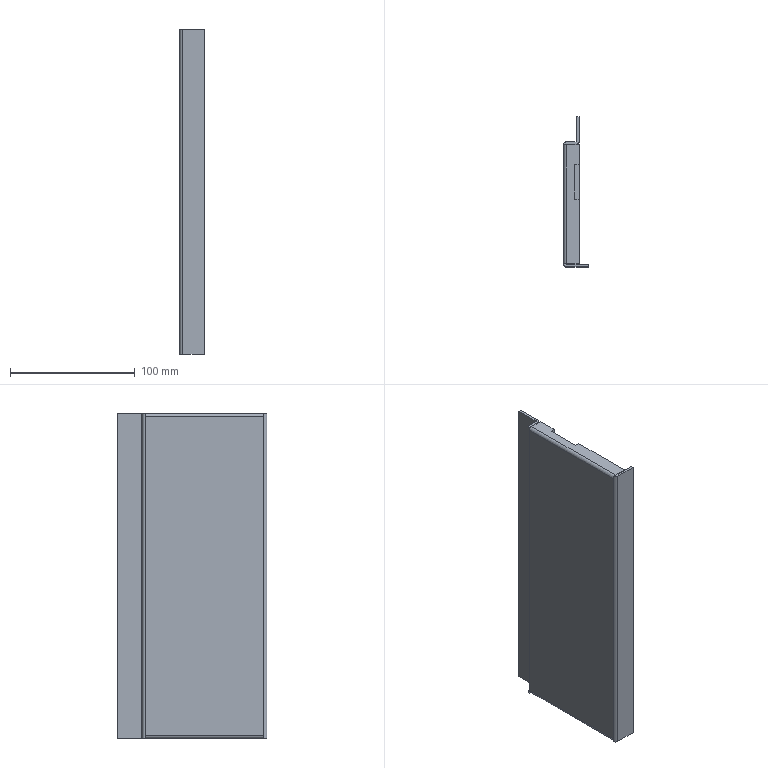Part | STEP file | Right Cover Plate | 1 solid | 42 faces | box 20 x 120 x 260 mm | volume 79765 mm3 | plane 32 | cylinder 10 | commonest cylinder face diameters 1 x5 5 x5
STEP:
#1=CARTESIAN_POINT('',(-10.5,-69.434,257.5));
#2=VERTEX_POINT('',#1);
#3=CARTESIAN_POINT('',(-10.5,-69.434,2.5));
#4=VERTEX_POINT('',#3);
#5=CARTESIAN_POINT('',(-10.5,-69.434,260.));
#6=DIRECTION('',(0.,0.,-1.));
#7=VECTOR('',#6,1000.);
#8=LINE('',#5,#7);
#9=EDGE_CURVE('',#2,#4,#8,.T.);
#10=ORIENTED_EDGE('',*,*,#9,.F.);
#11=CARTESIAN_POINT('',(-10.5,25.566,257.5));
#12=VERTEX_POINT('',#11);
#13=CARTESIAN_POINT('',(-10.5,28.066,257.5));
#14=DIRECTION('',(0.,-1.,0.));
#15=VECTOR('',#14,1000.);
#16=LINE('',#13,#15);
#17=EDGE_CURVE('',#12,#2,#16,.T.);
#18=ORIENTED_EDGE('',*,*,#17,.F.);
#19=CARTESIAN_POINT('',(-10.5,25.566,2.5));
#20=VERTEX_POINT('',#19);
#21=CARTESIAN_POINT('',(-10.5,25.566,260.));
#22=DIRECTION('',(0.,0.,1.));
#23=VECTOR('',#22,1000.);
#24=LINE('',#21,#23);
#25=EDGE_CURVE('',#20,#12,#24,.T.);
#26=ORIENTED_EDGE('',*,*,#25,.F.);
#27=CARTESIAN_POINT('',(-10.5,28.066,2.5));
#28=DIRECTION('',(0.,1.,0.));
#29=VECTOR('',#28,1000.);
#30=LINE('',#27,#29);
#31=EDGE_CURVE('',#4,#20,#30,.T.);
#32=ORIENTED_EDGE('',*,*,#31,.F.);
#33=EDGE_LOOP('',(#10,#18,#26,#32));
#34=FACE_OUTER_BOUND('',#33,.T.);
#35=CARTESIAN_POINT('',(-10.5,28.066,260.));
#36=DIRECTION('',(1.,0.,0.));
#37=DIRECTION('',(0.,1.,0.));
#38=AXIS2_PLACEMENT_3D('',#35,#36,#37);
#39=PLANE('',#38);
#40=ADVANCED_FACE('',(#34),#39,.F.);
#41=CARTESIAN_POINT('',(-8.5,-69.434,0.05051));
#42=VERTEX_POINT('',#41);
#43=CARTESIAN_POINT('',(-8.,-69.434,0.));
#44=VERTEX_POINT('',#43);
#45=CARTESIAN_POINT('',(-8.,-69.434,2.5));
#46=DIRECTION('',(0.,-1.,0.));
#47=DIRECTION('',(0.,0.,1.));
#48=AXIS2_PLACEMENT_3D('',#45,#46,#47);
#49=CIRCLE('',#48,2.5);
#50=EDGE_CURVE('',#42,#44,#49,.T.);
#51=ORIENTED_EDGE('',*,*,#50,.F.);
#52=CARTESIAN_POINT('',(-8.,-69.434,2.5));
#53=DIRECTION('',(0.,1.,0.));
#54=DIRECTION('',(0.,0.,1.));
#55=AXIS2_PLACEMENT_3D('',#52,#53,#54);
#56=CIRCLE('',#55,2.5);
#57=EDGE_CURVE('',#42,#4,#56,.T.);
#58=ORIENTED_EDGE('',*,*,#57,.T.);
#59=ORIENTED_EDGE('',*,*,#31,.T.);
#60=CARTESIAN_POINT('',(-8.5,25.566,0.05051));
#61=VERTEX_POINT('',#60);
#62=CARTESIAN_POINT('',(-8.,25.566,2.5));
#63=DIRECTION('',(0.,-1.,0.));
#64=DIRECTION('',(0.,0.,1.));
#65=AXIS2_PLACEMENT_3D('',#62,#63,#64);
#66=CIRCLE('',#65,2.5);
#67=EDGE_CURVE('',#20,#61,#66,.T.);
#68=ORIENTED_EDGE('',*,*,#67,.T.);
#69=CARTESIAN_POINT('',(-8.,25.566,0.));
#70=VERTEX_POINT('',#69);
#71=CARTESIAN_POINT('',(-8.,25.566,2.5));
#72=DIRECTION('',(0.,-1.,0.));
#73=DIRECTION('',(0.,0.,1.));
#74=AXIS2_PLACEMENT_3D('',#71,#72,#73);
#75=CIRCLE('',#74,2.5);
#76=EDGE_CURVE('',#61,#70,#75,.T.);
#77=ORIENTED_EDGE('',*,*,#76,.T.);
#78=CARTESIAN_POINT('',(-8.,25.566,0.));
#79=DIRECTION('',(0.,-1.,0.));
#80=VECTOR('',#79,1000.);
#81=LINE('',#78,#80);
#82=EDGE_CURVE('',#70,#44,#81,.T.);
#83=ORIENTED_EDGE('',*,*,#82,.T.);
#84=EDGE_LOOP('',(#51,#58,#59,#68,#77,#83));
#85=FACE_OUTER_BOUND('',#84,.T.);
#86=CARTESIAN_POINT('',(-8.,25.566,2.5));
#87=DIRECTION('',(0.,1.,0.));
#88=DIRECTION('',(0.,0.,1.));
#89=AXIS2_PLACEMENT_3D('',#86,#87,#88);
#90=CYLINDRICAL_SURFACE('',#89,2.5);
#91=ADVANCED_FACE('',(#85),#90,.T.);
#92=ORIENTED_EDGE('',*,*,#9,.T.);
#93=CARTESIAN_POINT('',(-10.5,-69.434,0.));
#94=VERTEX_POINT('',#93);
#95=CARTESIAN_POINT('',(-10.5,-69.434,260.));
#96=DIRECTION('',(0.,0.,-1.));
#97=VECTOR('',#96,1000.);
#98=LINE('',#95,#97);
#99=EDGE_CURVE('',#4,#94,#98,.T.);
#100=ORIENTED_EDGE('',*,*,#99,.T.);
#101=CARTESIAN_POINT('',(-8.,-71.934,0.));
#102=VERTEX_POINT('',#101);
#103=CARTESIAN_POINT('',(-8.,-69.434,0.));
#104=DIRECTION('',(0.,0.,1.));
#105=DIRECTION('',(-1.,0.,0.));
#106=AXIS2_PLACEMENT_3D('',#103,#104,#105);
#107=CIRCLE('',#106,2.5);
#108=EDGE_CURVE('',#94,#102,#107,.T.);
#109=ORIENTED_EDGE('',*,*,#108,.T.);
#110=CARTESIAN_POINT('',(-8.,-71.934,260.));
#111=VERTEX_POINT('',#110);
#112=CARTESIAN_POINT('',(-8.,-71.934,260.));
#113=DIRECTION('',(0.,0.,1.));
#114=VECTOR('',#113,1000.);
#115=LINE('',#112,#114);
#116=EDGE_CURVE('',#102,#111,#115,.T.);
#117=ORIENTED_EDGE('',*,*,#116,.T.);
#118=CARTESIAN_POINT('',(-10.5,-69.434,260.));
#119=VERTEX_POINT('',#118);
#120=CARTESIAN_POINT('',(-8.,-69.434,260.));
#121=DIRECTION('',(0.,0.,-1.));
#122=DIRECTION('',(-1.,0.,0.));
#123=AXIS2_PLACEMENT_3D('',#120,#121,#122);
#124=CIRCLE('',#123,2.5);
#125=EDGE_CURVE('',#111,#119,#124,.T.);
#126=ORIENTED_EDGE('',*,*,#125,.T.);
#127=CARTESIAN_POINT('',(-10.5,-69.434,260.));
#128=DIRECTION('',(0.,0.,-1.));
#129=VECTOR('',#128,1000.);
#130=LINE('',#127,#129);
#131=EDGE_CURVE('',#119,#2,#130,.T.);
#132=ORIENTED_EDGE('',*,*,#131,.T.);
#133=EDGE_LOOP('',(#92,#100,#109,#117,#126,#132));
#134=FACE_OUTER_BOUND('',#133,.T.);
#135=CARTESIAN_POINT('',(-8.,-69.434,260.));
#136=DIRECTION('',(0.,0.,-1.));
#137=DIRECTION('',(-1.,0.,0.));
#138=AXIS2_PLACEMENT_3D('',#135,#136,#137);
#139=CYLINDRICAL_SURFACE('',#138,2.5);
#140=ADVANCED_FACE('',(#134),#139,.T.);
#141=CARTESIAN_POINT('',(-8.5,25.566,259.949));
#142=VERTEX_POINT('',#141);
#143=CARTESIAN_POINT('',(-8.,25.566,260.));
#144=VERTEX_POINT('',#143);
#145=CARTESIAN_POINT('',(-8.,25.566,257.5));
#146=DIRECTION('',(0.,1.,0.));
#147=DIRECTION('',(0.,0.,-1.));
#148=AXIS2_PLACEMENT_3D('',#145,#146,#147);
#149=CIRCLE('',#148,2.5);
#150=EDGE_CURVE('',#142,#144,#149,.T.);
#151=ORIENTED_EDGE('',*,*,#150,.F.);
#152=CARTESIAN_POINT('',(-8.,25.566,257.5));
#153=DIRECTION('',(0.,-1.,0.));
#154=DIRECTION('',(0.,0.,-1.));
#155=AXIS2_PLACEMENT_3D('',#152,#153,#154);
#156=CIRCLE('',#155,2.5);
#157=EDGE_CURVE('',#142,#12,#156,.T.);
#158=ORIENTED_EDGE('',*,*,#157,.T.);
#159=ORIENTED_EDGE('',*,*,#17,.T.);
#160=CARTESIAN_POINT('',(-8.5,-69.434,259.949));
#161=VERTEX_POINT('',#160);
#162=CARTESIAN_POINT('',(-8.,-69.434,257.5));
#163=DIRECTION('',(0.,1.,0.));
#164=DIRECTION('',(0.,0.,-1.));
#165=AXIS2_PLACEMENT_3D('',#162,#163,#164);
#166=CIRCLE('',#165,2.5);
#167=EDGE_CURVE('',#2,#161,#166,.T.);
#168=ORIENTED_EDGE('',*,*,#167,.T.);
#169=CARTESIAN_POINT('',(-8.,-69.434,260.));
#170=VERTEX_POINT('',#169);
#171=CARTESIAN_POINT('',(-8.,-69.434,257.5));
#172=DIRECTION('',(0.,1.,0.));
#173=DIRECTION('',(0.,0.,-1.));
#174=AXIS2_PLACEMENT_3D('',#171,#172,#173);
#175=CIRCLE('',#174,2.5);
#176=EDGE_CURVE('',#161,#170,#175,.T.);
#177=ORIENTED_EDGE('',*,*,#176,.T.);
#178=CARTESIAN_POINT('',(-8.,-69.434,260.));
#179=DIRECTION('',(0.,1.,0.));
#180=VECTOR('',#179,1000.);
#181=LINE('',#178,#180);
#182=EDGE_CURVE('',#170,#144,#181,.T.);
#183=ORIENTED_EDGE('',*,*,#182,.T.);
#184=EDGE_LOOP('',(#151,#158,#159,#168,#177,#183));
#185=FACE_OUTER_BOUND('',#184,.T.);
#186=CARTESIAN_POINT('',(-8.,-69.434,257.5));
#187=DIRECTION('',(0.,-1.,0.));
#188=DIRECTION('',(0.,0.,-1.));
#189=AXIS2_PLACEMENT_3D('',#186,#187,#188);
#190=CYLINDRICAL_SURFACE('',#189,2.5);
#191=ADVANCED_FACE('',(#185),#190,.T.);
#192=CARTESIAN_POINT('',(-10.5,25.566,260.));
#193=VERTEX_POINT('',#192);
#194=CARTESIAN_POINT('',(-8.,28.066,260.));
#195=VERTEX_POINT('',#194);
#196=CARTESIAN_POINT('',(-8.,25.566,260.));
#197=DIRECTION('',(0.,0.,-1.));
#198=DIRECTION('',(-1.,0.,0.));
#199=AXIS2_PLACEMENT_3D('',#196,#197,#198);
#200=CIRCLE('',#199,2.5);
#201=EDGE_CURVE('',#193,#195,#200,.T.);
#202=ORIENTED_EDGE('',*,*,#201,.T.);
#203=CARTESIAN_POINT('',(-8.,28.066,0.));
#204=VERTEX_POINT('',#203);
#205=CARTESIAN_POINT('',(-8.,28.066,260.));
#206=DIRECTION('',(0.,0.,-1.));
#207=VECTOR('',#206,1000.);
#208=LINE('',#205,#207);
#209=EDGE_CURVE('',#195,#204,#208,.T.);
#210=ORIENTED_EDGE('',*,*,#209,.T.);
#211=CARTESIAN_POINT('',(-10.5,25.566,0.));
#212=VERTEX_POINT('',#211);
#213=CARTESIAN_POINT('',(-8.,25.566,0.));
#214=DIRECTION('',(0.,0.,1.));
#215=DIRECTION('',(-1.,0.,0.));
#216=AXIS2_PLACEMENT_3D('',#213,#214,#215);
#217=CIRCLE('',#216,2.5);
#218=EDGE_CURVE('',#204,#212,#217,.T.);
#219=ORIENTED_EDGE('',*,*,#218,.T.);
#220=CARTESIAN_POINT('',(-10.5,25.566,260.));
#221=DIRECTION('',(0.,0.,1.));
#222=VECTOR('',#221,1000.);
#223=LINE('',#220,#222);
#224=EDGE_CURVE('',#212,#20,#223,.T.);
#225=ORIENTED_EDGE('',*,*,#224,.T.);
#226=ORIENTED_EDGE('',*,*,#25,.T.);
#227=CARTESIAN_POINT('',(-10.5,25.566,260.));
#228=DIRECTION('',(0.,0.,1.));
#229=VECTOR('',#228,1000.);
#230=LINE('',#227,#229);
#231=EDGE_CURVE('',#12,#193,#230,.T.);
#232=ORIENTED_EDGE('',*,*,#231,.T.);
#233=EDGE_LOOP('',(#202,#210,#219,#225,#226,#232));
#234=FACE_OUTER_BOUND('',#233,.T.);
#235=CARTESIAN_POINT('',(-8.,25.566,260.));
#236=DIRECTION('',(0.,0.,-1.));
#237=DIRECTION('',(-1.,0.,0.));
#238=AXIS2_PLACEMENT_3D('',#235,#236,#237);
#239=CYLINDRICAL_SURFACE('',#238,2.5);
#240=ADVANCED_FACE('',(#234),#239,.T.);
#241=CARTESIAN_POINT('',(-8.5,-69.434,0.));
#242=VERTEX_POINT('',#241);
#243=CARTESIAN_POINT('',(-8.5,-69.434,260.));
#244=DIRECTION('',(0.,0.,-1.));
#245=VECTOR('',#244,1000.);
#246=LINE('',#243,#245);
#247=EDGE_CURVE('',#42,#242,#246,.T.);
#248=ORIENTED_EDGE('',*,*,#247,.T.);
#249=CARTESIAN_POINT('',(-8.5,-69.434,0.));
#250=DIRECTION('',(-1.,0.,0.));
#251=VECTOR('',#250,1000.);
#252=LINE('',#249,#251);
#253=EDGE_CURVE('',#242,#94,#252,.T.);
#254=ORIENTED_EDGE('',*,*,#253,.T.);
#255=ORIENTED_EDGE('',*,*,#99,.F.);
#256=ORIENTED_EDGE('',*,*,#57,.F.);
#257=EDGE_LOOP('',(#248,#254,#255,#256));
#258=FACE_OUTER_BOUND('',#257,.T.);
#259=CARTESIAN_POINT('',(-8.5,-69.434,2.5));
#260=DIRECTION('',(0.,1.,0.));
#261=DIRECTION('',(-1.,0.,0.));
#262=AXIS2_PLACEMENT_3D('',#259,#260,#261);
#263=PLANE('',#262);
#264=ADVANCED_FACE('',(#258),#263,.T.);
#265=CARTESIAN_POINT('',(2.,25.566,0.));
#266=VERTEX_POINT('',#265);
#267=CARTESIAN_POINT('',(0.,25.566,0.));
#268=DIRECTION('',(-1.,0.,0.));
#269=VECTOR('',#268,1000.);
#270=LINE('',#267,#269);
#271=EDGE_CURVE('',#266,#70,#270,.T.);
#272=ORIENTED_EDGE('',*,*,#271,.F.);
#273=CARTESIAN_POINT('',(2.,-69.434,0.));
#274=VERTEX_POINT('',#273);
#275=CARTESIAN_POINT('',(2.,0.,0.));
#276=DIRECTION('',(0.,1.,0.));
#277=VECTOR('',#276,1000.);
#278=LINE('',#275,#277);
#279=EDGE_CURVE('',#274,#266,#278,.T.);
#280=ORIENTED_EDGE('',*,*,#279,.F.);
#281=CARTESIAN_POINT('',(0.,-69.434,0.));
#282=DIRECTION('',(1.,0.,0.));
#283=VECTOR('',#282,1000.);
#284=LINE('',#281,#283);
#285=EDGE_CURVE('',#44,#274,#284,.T.);
#286=ORIENTED_EDGE('',*,*,#285,.F.);
#287=ORIENTED_EDGE('',*,*,#82,.F.);
#288=EDGE_LOOP('',(#272,#280,#286,#287));
#289=FACE_OUTER_BOUND('',#288,.T.);
#290=CARTESIAN_POINT('',(0.,0.,0.));
#291=DIRECTION('',(0.,0.,1.));
#292=DIRECTION('',(1.,0.,0.));
#293=AXIS2_PLACEMENT_3D('',#290,#291,#292);
#294=PLANE('',#293);
#295=ADVANCED_FACE('',(#289),#294,.F.);
#296=ORIENTED_EDGE('',*,*,#224,.F.);
#297=CARTESIAN_POINT('',(-8.5,25.566,0.));
#298=VERTEX_POINT('',#297);
#299=CARTESIAN_POINT('',(-8.5,25.566,0.));
#300=DIRECTION('',(1.,0.,0.));
#301=VECTOR('',#300,1000.);
#302=LINE('',#299,#301);
#303=EDGE_CURVE('',#212,#298,#302,.T.);
#304=ORIENTED_EDGE('',*,*,#303,.T.);
#305=CARTESIAN_POINT('',(-8.5,25.566,260.));
#306=DIRECTION('',(0.,0.,1.));
#307=VECTOR('',#306,1000.);
#308=LINE('',#305,#307);
#309=EDGE_CURVE('',#298,#61,#308,.T.);
#310=ORIENTED_EDGE('',*,*,#309,.T.);
#311=ORIENTED_EDGE('',*,*,#67,.F.);
#312=EDGE_LOOP('',(#296,#304,#310,#311));
#313=FACE_OUTER_BOUND('',#312,.T.);
#314=CARTESIAN_POINT('',(-8.5,25.566,0.));
#315=DIRECTION('',(0.,-1.,0.));
#316=DIRECTION('',(1.,0.,0.));
#317=AXIS2_PLACEMENT_3D('',#314,#315,#316);
#318=PLANE('',#317);
#319=ADVANCED_FACE('',(#313),#318,.T.);
#320=ORIENTED_EDGE('',*,*,#131,.F.);
#321=CARTESIAN_POINT('',(-8.5,-69.434,260.));
#322=VERTEX_POINT('',#321);
#323=CARTESIAN_POINT('',(-8.5,-69.434,260.));
#324=DIRECTION('',(1.,0.,0.));
#325=VECTOR('',#324,1000.);
#326=LINE('',#323,#325);
#327=EDGE_CURVE('',#119,#322,#326,.T.);
#328=ORIENTED_EDGE('',*,*,#327,.T.);
#329=CARTESIAN_POINT('',(-8.5,-69.434,260.));
#330=DIRECTION('',(0.,0.,-1.));
#331=VECTOR('',#330,1000.);
#332=LINE('',#329,#331);
#333=EDGE_CURVE('',#322,#161,#332,.T.);
#334=ORIENTED_EDGE('',*,*,#333,.T.);
#335=ORIENTED_EDGE('',*,*,#167,.F.);
#336=EDGE_LOOP('',(#320,#328,#334,#335));
#337=FACE_OUTER_BOUND('',#336,.T.);
#338=CARTESIAN_POINT('',(-8.5,-69.434,260.));
#339=DIRECTION('',(0.,1.,0.));
#340=DIRECTION('',(-1.,0.,0.));
#341=AXIS2_PLACEMENT_3D('',#338,#339,#340);
#342=PLANE('',#341);
#343=ADVANCED_FACE('',(#337),#342,.T.);
#344=ORIENTED_EDGE('',*,*,#125,.F.);
#345=CARTESIAN_POINT('',(9.5,-71.934,260.));
#346=VERTEX_POINT('',#345);
#347=CARTESIAN_POINT('',(-10.5,-71.934,260.));
#348=DIRECTION('',(1.,0.,0.));
#349=VECTOR('',#348,1000.);
#350=LINE('',#347,#349);
#351=EDGE_CURVE('',#111,#346,#350,.T.);
#352=ORIENTED_EDGE('',*,*,#351,.T.);
#353=CARTESIAN_POINT('',(9.5,-69.934,260.));
#354=VERTEX_POINT('',#353);
#355=CARTESIAN_POINT('',(9.5,-69.434,260.));
#356=DIRECTION('',(0.,1.,0.));
#357=VECTOR('',#356,1000.);
#358=LINE('',#355,#357);
#359=EDGE_CURVE('',#346,#354,#358,.T.);
#360=ORIENTED_EDGE('',*,*,#359,.T.);
#361=CARTESIAN_POINT('',(-8.,-69.934,260.));
#362=VERTEX_POINT('',#361);
#363=CARTESIAN_POINT('',(-8.,-69.934,260.));
#364=DIRECTION('',(-1.,0.,0.));
#365=VECTOR('',#364,1000.);
#366=LINE('',#363,#365);
#367=EDGE_CURVE('',#354,#362,#366,.T.);
#368=ORIENTED_EDGE('',*,*,#367,.T.);
#369=CARTESIAN_POINT('',(-8.,-69.434,260.));
#370=DIRECTION('',(0.,0.,-1.));
#371=DIRECTION('',(-1.,0.,0.));
#372=AXIS2_PLACEMENT_3D('',#369,#370,#371);
#373=CIRCLE('',#372,0.5);
#374=EDGE_CURVE('',#362,#322,#373,.T.);
#375=ORIENTED_EDGE('',*,*,#374,.T.);
#376=ORIENTED_EDGE('',*,*,#327,.F.);
#377=EDGE_LOOP('',(#344,#352,#360,#368,#375,#376));
#378=FACE_OUTER_BOUND('',#377,.T.);
#379=CARTESIAN_POINT('',(-10.5,-69.434,260.));
#380=DIRECTION('',(0.,0.,1.));
#381=DIRECTION('',(1.,0.,0.));
#382=AXIS2_PLACEMENT_3D('',#379,#380,#381);
#383=PLANE('',#382);
#384=ADVANCED_FACE('',(#378),#383,.T.);
#385=CARTESIAN_POINT('',(9.5,-71.934,0.));
#386=VERTEX_POINT('',#385);
#387=CARTESIAN_POINT('',(9.5,-71.934,260.));
#388=DIRECTION('',(0.,0.,-1.));
#389=VECTOR('',#388,1000.);
#390=LINE('',#387,#389);
#391=EDGE_CURVE('',#346,#386,#390,.T.);
#392=ORIENTED_EDGE('',*,*,#391,.F.);
#393=ORIENTED_EDGE('',*,*,#351,.F.);
#394=ORIENTED_EDGE('',*,*,#116,.F.);
#395=CARTESIAN_POINT('',(-10.5,-71.934,0.));
#396=DIRECTION('',(-1.,0.,0.));
#397=VECTOR('',#396,1000.);
#398=LINE('',#395,#397);
#399=EDGE_CURVE('',#386,#102,#398,.T.);
#400=ORIENTED_EDGE('',*,*,#399,.F.);
#401=EDGE_LOOP('',(#392,#393,#394,#400));
#402=FACE_OUTER_BOUND('',#401,.T.);
#403=CARTESIAN_POINT('',(-10.5,-71.934,260.));
#404=DIRECTION('',(0.,1.,0.));
#405=DIRECTION('',(0.,0.,1.));
#406=AXIS2_PLACEMENT_3D('',#403,#404,#405);
#407=PLANE('',#406);
#408=ADVANCED_FACE('',(#402),#407,.F.);
#409=ORIENTED_EDGE('',*,*,#253,.F.);
#410=CARTESIAN_POINT('',(-8.,-69.934,0.));
#411=VERTEX_POINT('',#410);
#412=CARTESIAN_POINT('',(-8.,-69.434,0.));
#413=DIRECTION('',(0.,0.,1.));
#414=DIRECTION('',(-1.,0.,0.));
#415=AXIS2_PLACEMENT_3D('',#412,#413,#414);
#416=CIRCLE('',#415,0.5);
#417=EDGE_CURVE('',#242,#411,#416,.T.);
#418=ORIENTED_EDGE('',*,*,#417,.T.);
#419=CARTESIAN_POINT('',(9.5,-69.934,0.));
#420=VERTEX_POINT('',#419);
#421=CARTESIAN_POINT('',(-8.5,-69.934,0.));
#422=DIRECTION('',(1.,0.,0.));
#423=VECTOR('',#422,1000.);
#424=LINE('',#421,#423);
#425=EDGE_CURVE('',#411,#420,#424,.T.);
#426=ORIENTED_EDGE('',*,*,#425,.T.);
#427=CARTESIAN_POINT('',(9.5,-69.434,0.));
#428=DIRECTION('',(0.,-1.,0.));
#429=VECTOR('',#428,1000.);
#430=LINE('',#427,#429);
#431=EDGE_CURVE('',#420,#386,#430,.T.);
#432=ORIENTED_EDGE('',*,*,#431,.T.);
#433=ORIENTED_EDGE('',*,*,#399,.T.);
#434=ORIENTED_EDGE('',*,*,#108,.F.);
#435=EDGE_LOOP('',(#409,#418,#426,#432,#433,#434));
#436=FACE_OUTER_BOUND('',#435,.T.);
#437=CARTESIAN_POINT('',(-8.,-71.934,0.));
#438=DIRECTION('',(0.,0.,-1.));
#439=DIRECTION('',(-1.,0.,0.));
#440=AXIS2_PLACEMENT_3D('',#437,#438,#439);
#441=PLANE('',#440);
#442=ADVANCED_FACE('',(#436),#441,.T.);
#443=CARTESIAN_POINT('',(-8.5,25.566,260.));
#444=VERTEX_POINT('',#443);
#445=CARTESIAN_POINT('',(-8.5,25.566,260.));
#446=DIRECTION('',(0.,0.,1.));
#447=VECTOR('',#446,1000.);
#448=LINE('',#445,#447);
#449=EDGE_CURVE('',#142,#444,#448,.T.);
#450=ORIENTED_EDGE('',*,*,#449,.T.);
#451=CARTESIAN_POINT('',(-8.5,25.566,260.));
#452=DIRECTION('',(-1.,0.,0.));
#453=VECTOR('',#452,1000.);
#454=LINE('',#451,#453);
#455=EDGE_CURVE('',#444,#193,#454,.T.);
#456=ORIENTED_EDGE('',*,*,#455,.T.);
#457=ORIENTED_EDGE('',*,*,#231,.F.);
#458=ORIENTED_EDGE('',*,*,#157,.F.);
#459=EDGE_LOOP('',(#450,#456,#457,#458));
#460=FACE_OUTER_BOUND('',#459,.T.);
#461=CARTESIAN_POINT('',(-8.5,25.566,257.5));
#462=DIRECTION('',(0.,-1.,0.));
#463=DIRECTION('',(1.,0.,0.));
#464=AXIS2_PLACEMENT_3D('',#461,#462,#463);
#465=PLANE('',#464);
#466=ADVANCED_FACE('',(#460),#465,.T.);
#467=CARTESIAN_POINT('',(2.,-69.434,260.));
#468=VERTEX_POINT('',#467);
#469=CARTESIAN_POINT('',(0.,-69.434,260.));
#470=DIRECTION('',(1.,0.,0.));
#471=VECTOR('',#470,1000.);
#472=LINE('',#469,#471);
#473=EDGE_CURVE('',#170,#468,#472,.T.);
#474=ORIENTED_EDGE('',*,*,#473,.T.);
#475=CARTESIAN_POINT('',(2.,-17.934,260.));
#476=VERTEX_POINT('',#475);
#477=CARTESIAN_POINT('',(2.,0.,260.));
#478=DIRECTION('',(0.,1.,0.));
#479=VECTOR('',#478,1000.);
#480=LINE('',#477,#479);
#481=EDGE_CURVE('',#468,#476,#480,.T.);
#482=ORIENTED_EDGE('',*,*,#481,.T.);
#483=CARTESIAN_POINT('',(-1.5,-17.934,260.));
#484=VERTEX_POINT('',#483);
#485=CARTESIAN_POINT('',(0.,-17.934,260.));
#486=DIRECTION('',(-1.,0.,0.));
#487=VECTOR('',#486,1000.);
#488=LINE('',#485,#487);
#489=EDGE_CURVE('',#476,#484,#488,.T.);
#490=ORIENTED_EDGE('',*,*,#489,.T.);
#491=CARTESIAN_POINT('',(-1.5,10.066,260.));
#492=VERTEX_POINT('',#491);
#493=CARTESIAN_POINT('',(-1.5,0.,260.));
#494=DIRECTION('',(0.,1.,0.));
#495=VECTOR('',#494,1000.);
#496=LINE('',#493,#495);
#497=EDGE_CURVE('',#484,#492,#496,.T.);
#498=ORIENTED_EDGE('',*,*,#497,.T.);
#499=CARTESIAN_POINT('',(2.,10.066,260.));
#500=VERTEX_POINT('',#499);
#501=CARTESIAN_POINT('',(0.,10.066,260.));
#502=DIRECTION('',(1.,0.,0.));
#503=VECTOR('',#502,1000.);
#504=LINE('',#501,#503);
#505=EDGE_CURVE('',#492,#500,#504,.T.);
#506=ORIENTED_EDGE('',*,*,#505,.T.);
#507=CARTESIAN_POINT('',(2.,25.566,260.));
#508=VERTEX_POINT('',#507);
#509=CARTESIAN_POINT('',(2.,0.,260.));
#510=DIRECTION('',(0.,1.,0.));
#511=VECTOR('',#510,1000.);
#512=LINE('',#509,#511);
#513=EDGE_CURVE('',#500,#508,#512,.T.);
#514=ORIENTED_EDGE('',*,*,#513,.T.);
#515=CARTESIAN_POINT('',(0.,25.566,260.));
#516=DIRECTION('',(-1.,0.,0.));
#517=VECTOR('',#516,1000.);
#518=LINE('',#515,#517);
#519=EDGE_CURVE('',#508,#144,#518,.T.);
#520=ORIENTED_EDGE('',*,*,#519,.T.);
#521=ORIENTED_EDGE('',*,*,#182,.F.);
#522=EDGE_LOOP('',(#474,#482,#490,#498,#506,#514,#520,#521));
#523=FACE_OUTER_BOUND('',#522,.T.);
#524=CARTESIAN_POINT('',(0.,0.,260.));
#525=DIRECTION('',(0.,0.,1.));
#526=DIRECTION('',(1.,0.,0.));
#527=AXIS2_PLACEMENT_3D('',#524,#525,#526);
#528=PLANE('',#527);
#529=ADVANCED_FACE('',(#523),#528,.T.);
#530=ORIENTED_EDGE('',*,*,#209,.F.);
#531=CARTESIAN_POINT('',(-0.5,28.066,260.));
#532=VERTEX_POINT('',#531);
#533=CARTESIAN_POINT('',(0.,28.066,260.));
#534=DIRECTION('',(-1.,0.,0.));
#535=VECTOR('',#534,1000.);
#536=LINE('',#533,#535);
#537=EDGE_CURVE('',#532,#195,#536,.T.);
#538=ORIENTED_EDGE('',*,*,#537,.F.);
#539=CARTESIAN_POINT('',(-0.5,28.066,0.));
#540=VERTEX_POINT('',#539);
#541=CARTESIAN_POINT('',(-0.5,28.066,260.));
#542=DIRECTION('',(0.,0.,1.));
#543=VECTOR('',#542,1000.);
#544=LINE('',#541,#543);
#545=EDGE_CURVE('',#540,#532,#544,.T.);
#546=ORIENTED_EDGE('',*,*,#545,.F.);
#547=CARTESIAN_POINT('',(0.,28.066,0.));
#548=DIRECTION('',(1.,0.,0.));
#549=VECTOR('',#548,1000.);
#550=LINE('',#547,#549);
#551=EDGE_CURVE('',#204,#540,#550,.T.);
#552=ORIENTED_EDGE('',*,*,#551,.F.);
#553=EDGE_LOOP('',(#530,#538,#546,#552));
#554=FACE_OUTER_BOUND('',#553,.T.);
#555=CARTESIAN_POINT('',(0.,28.066,260.));
#556=DIRECTION('',(0.,-1.,0.));
#557=DIRECTION('',(0.,0.,-1.));
#558=AXIS2_PLACEMENT_3D('',#555,#556,#557);
#559=PLANE('',#558);
#560=ADVANCED_FACE('',(#554),#559,.F.);
#561=ORIENTED_EDGE('',*,*,#455,.F.);
#562=CARTESIAN_POINT('',(-8.,26.066,260.));
#563=VERTEX_POINT('',#562);
#564=CARTESIAN_POINT('',(-8.,25.566,260.));
#565=DIRECTION('',(0.,0.,-1.));
#566=DIRECTION('',(-1.,0.,0.));
#567=AXIS2_PLACEMENT_3D('',#564,#565,#566);
#568=CIRCLE('',#567,0.5);
#569=EDGE_CURVE('',#444,#563,#568,.T.);
#570=ORIENTED_EDGE('',*,*,#569,.T.);
#571=CARTESIAN_POINT('',(-0.5,26.066,260.));
#572=VERTEX_POINT('',#571);
#573=CARTESIAN_POINT('',(-8.5,26.066,260.));
#574=DIRECTION('',(1.,0.,0.));
#575=VECTOR('',#574,1000.);
#576=LINE('',#573,#575);
#577=EDGE_CURVE('',#563,#572,#576,.T.);
#578=ORIENTED_EDGE('',*,*,#577,.T.);
#579=CARTESIAN_POINT('',(2.,28.566,260.));
#580=VERTEX_POINT('',#579);
#581=CARTESIAN_POINT('',(-0.5,28.566,260.));
#582=DIRECTION('',(0.,0.,1.));
#583=DIRECTION('',(-1.,0.,0.));
#584=AXIS2_PLACEMENT_3D('',#581,#582,#583);
#585=CIRCLE('',#584,2.5);
#586=EDGE_CURVE('',#572,#580,#585,.T.);
#587=ORIENTED_EDGE('',*,*,#586,.T.);
#588=CARTESIAN_POINT('',(2.,48.066,260.));
#589=VERTEX_POINT('',#588);
#590=CARTESIAN_POINT('',(2.,26.066,260.));
#591=DIRECTION('',(0.,1.,0.));
#592=VECTOR('',#591,1000.);
#593=LINE('',#590,#592);
#594=EDGE_CURVE('',#580,#589,#593,.T.);
#595=ORIENTED_EDGE('',*,*,#594,.T.);
#596=CARTESIAN_POINT('',(0.,48.066,260.));
#597=VERTEX_POINT('',#596);
#598=CARTESIAN_POINT('',(-0.5,48.066,260.));
#599=DIRECTION('',(-1.,0.,0.));
#600=VECTOR('',#599,1000.);
#601=LINE('',#598,#600);
#602=EDGE_CURVE('',#589,#597,#601,.T.);
#603=ORIENTED_EDGE('',*,*,#602,.T.);
#604=CARTESIAN_POINT('',(0.,28.566,260.));
#605=VERTEX_POINT('',#604);
#606=CARTESIAN_POINT('',(0.,48.066,260.));
#607=DIRECTION('',(0.,-1.,0.));
#608=VECTOR('',#607,1000.);
#609=LINE('',#606,#608);
#610=EDGE_CURVE('',#597,#605,#609,.T.);
#611=ORIENTED_EDGE('',*,*,#610,.T.);
#612=CARTESIAN_POINT('',(-0.5,28.566,260.));
#613=DIRECTION('',(0.,0.,-1.));
#614=DIRECTION('',(-1.,0.,0.));
#615=AXIS2_PLACEMENT_3D('',#612,#613,#614);
#616=CIRCLE('',#615,0.5);
#617=EDGE_CURVE('',#605,#532,#616,.T.);
#618=ORIENTED_EDGE('',*,*,#617,.T.);
#619=ORIENTED_EDGE('',*,*,#537,.T.);
#620=ORIENTED_EDGE('',*,*,#201,.F.);
#621=EDGE_LOOP('',(#561,#570,#578,#587,#595,#603,#611,#618,#619,#620));
#622=FACE_OUTER_BOUND('',#621,.T.);
#623=CARTESIAN_POINT('',(-8.,28.066,260.));
#624=DIRECTION('',(0.,0.,1.));
#625=DIRECTION('',(1.,0.,0.));
#626=AXIS2_PLACEMENT_3D('',#623,#624,#625);
#627=PLANE('',#626);
#628=ADVANCED_FACE('',(#622),#627,.T.);
#629=ORIENTED_EDGE('',*,*,#218,.F.);
#630=ORIENTED_EDGE('',*,*,#551,.T.);
#631=CARTESIAN_POINT('',(0.,28.566,0.));
#632=VERTEX_POINT('',#631);
#633=CARTESIAN_POINT('',(-0.5,28.566,0.));
#634=DIRECTION('',(0.,0.,1.));
#635=DIRECTION('',(-1.,0.,0.));
#636=AXIS2_PLACEMENT_3D('',#633,#634,#635);
#637=CIRCLE('',#636,0.5);
#638=EDGE_CURVE('',#540,#632,#637,.T.);
#639=ORIENTED_EDGE('',*,*,#638,.T.);
#640=CARTESIAN_POINT('',(0.,48.066,0.));
#641=VERTEX_POINT('',#640);
#642=CARTESIAN_POINT('',(0.,48.066,0.));
#643=DIRECTION('',(0.,1.,0.));
#644=VECTOR('',#643,1000.);
#645=LINE('',#642,#644);
#646=EDGE_CURVE('',#632,#641,#645,.T.);
#647=ORIENTED_EDGE('',*,*,#646,.T.);
#648=CARTESIAN_POINT('',(2.,48.066,0.));
#649=VERTEX_POINT('',#648);
#650=CARTESIAN_POINT('',(-8.,48.066,0.));
#651=DIRECTION('',(-1.,0.,0.));
#652=VECTOR('',#651,1000.);
#653=LINE('',#650,#652);
#654=EDGE_CURVE('',#649,#641,#653,.T.);
#655=ORIENTED_EDGE('',*,*,#654,.F.);
#656=CARTESIAN_POINT('',(2.,28.566,0.));
#657=VERTEX_POINT('',#656);
#658=CARTESIAN_POINT('',(2.,-69.434,0.));
#659=DIRECTION('',(0.,1.,0.));
#660=VECTOR('',#659,1000.);
#661=LINE('',#658,#660);
#662=EDGE_CURVE('',#657,#649,#661,.T.);
#663=ORIENTED_EDGE('',*,*,#662,.F.);
#664=CARTESIAN_POINT('',(-0.5,26.066,0.));
#665=VERTEX_POINT('',#664);
#666=CARTESIAN_POINT('',(-0.5,28.566,0.));
#667=DIRECTION('',(0.,0.,-1.));
#668=DIRECTION('',(-1.,0.,0.));
#669=AXIS2_PLACEMENT_3D('',#666,#667,#668);
#670=CIRCLE('',#669,2.5);
#671=EDGE_CURVE('',#657,#665,#670,.T.);
#672=ORIENTED_EDGE('',*,*,#671,.T.);
#673=CARTESIAN_POINT('',(-8.,26.066,0.));
#674=VERTEX_POINT('',#673);
#675=CARTESIAN_POINT('',(2.,26.066,0.));
#676=DIRECTION('',(-1.,0.,0.));
#677=VECTOR('',#676,1000.);
#678=LINE('',#675,#677);
#679=EDGE_CURVE('',#665,#674,#678,.T.);
#680=ORIENTED_EDGE('',*,*,#679,.T.);
#681=CARTESIAN_POINT('',(-8.,25.566,0.));
#682=DIRECTION('',(0.,0.,1.));
#683=DIRECTION('',(-1.,0.,0.));
#684=AXIS2_PLACEMENT_3D('',#681,#682,#683);
#685=CIRCLE('',#684,0.5);
#686=EDGE_CURVE('',#674,#298,#685,.T.);
#687=ORIENTED_EDGE('',*,*,#686,.T.);
#688=ORIENTED_EDGE('',*,*,#303,.F.);
#689=EDGE_LOOP('',(#629,#630,#639,#647,#655,#663,#672,#680,#687,#688));
#690=FACE_OUTER_BOUND('',#689,.T.);
#691=CARTESIAN_POINT('',(-10.5,25.566,0.));
#692=DIRECTION('',(0.,0.,-1.));
#693=DIRECTION('',(-1.,0.,0.));
#694=AXIS2_PLACEMENT_3D('',#691,#692,#693);
#695=PLANE('',#694);
#696=ADVANCED_FACE('',(#690),#695,.T.);
#697=CARTESIAN_POINT('',(-8.,25.566,2.));
#698=VERTEX_POINT('',#697);
#699=CARTESIAN_POINT('',(2.,25.566,2.));
#700=VERTEX_POINT('',#699);
#701=CARTESIAN_POINT('',(2.,25.566,2.));
#702=DIRECTION('',(1.,0.,0.));
#703=VECTOR('',#702,1000.);
#704=LINE('',#701,#703);
#705=EDGE_CURVE('',#698,#700,#704,.T.);
#706=ORIENTED_EDGE('',*,*,#705,.T.);
#707=CARTESIAN_POINT('',(2.,25.566,0.));
#708=DIRECTION('',(0.,0.,-1.));
#709=VECTOR('',#708,1000.);
#710=LINE('',#707,#709);
#711=EDGE_CURVE('',#700,#266,#710,.T.);
#712=ORIENTED_EDGE('',*,*,#711,.T.);
#713=ORIENTED_EDGE('',*,*,#271,.T.);
#714=ORIENTED_EDGE('',*,*,#76,.F.);
#715=CARTESIAN_POINT('',(-8.5,25.566,2.5));
#716=VERTEX_POINT('',#715);
#717=CARTESIAN_POINT('',(-8.5,25.566,2.5));
#718=DIRECTION('',(0.,0.,-1.));
#719=VECTOR('',#718,1000.);
#720=LINE('',#717,#719);
#721=EDGE_CURVE('',#716,#61,#720,.T.);
#722=ORIENTED_EDGE('',*,*,#721,.F.);
#723=CARTESIAN_POINT('',(-8.,25.566,2.5));
#724=DIRECTION('',(0.,1.,0.));
#725=DIRECTION('',(0.,0.,1.));
#726=AXIS2_PLACEMENT_3D('',#723,#724,#725);
#727=CIRCLE('',#726,0.5);
#728=EDGE_CURVE('',#698,#716,#727,.T.);
#729=ORIENTED_EDGE('',*,*,#728,.F.);
#730=EDGE_LOOP('',(#706,#712,#713,#714,#722,#729));
#731=FACE_OUTER_BOUND('',#730,.T.);
#732=CARTESIAN_POINT('',(2.,25.566,0.));
#733=DIRECTION('',(0.,1.,0.));
#734=DIRECTION('',(0.,0.,1.));
#735=AXIS2_PLACEMENT_3D('',#732,#733,#734);
#736=PLANE('',#735);
#737=ADVANCED_FACE('',(#731),#736,.T.);
#738=ORIENTED_EDGE('',*,*,#279,.T.);
#739=ORIENTED_EDGE('',*,*,#711,.F.);
#740=CARTESIAN_POINT('',(2.,-69.434,2.));
#741=VERTEX_POINT('',#740);
#742=CARTESIAN_POINT('',(2.,-69.434,2.));
#743=DIRECTION('',(0.,-1.,0.));
#744=VECTOR('',#743,1000.);
#745=LINE('',#742,#744);
#746=EDGE_CURVE('',#700,#741,#745,.T.);
#747=ORIENTED_EDGE('',*,*,#746,.T.);
#748=CARTESIAN_POINT('',(2.,-69.434,0.));
#749=DIRECTION('',(0.,0.,-1.));
#750=VECTOR('',#749,1000.);
#751=LINE('',#748,#750);
#752=EDGE_CURVE('',#741,#274,#751,.T.);
#753=ORIENTED_EDGE('',*,*,#752,.T.);
#754=EDGE_LOOP('',(#738,#739,#747,#753));
#755=FACE_OUTER_BOUND('',#754,.T.);
#756=CARTESIAN_POINT('',(2.,-69.434,0.));
#757=DIRECTION('',(1.,0.,0.));
#758=DIRECTION('',(0.,0.,-1.));
#759=AXIS2_PLACEMENT_3D('',#756,#757,#758);
#760=PLANE('',#759);
#761=ADVANCED_FACE('',(#755),#760,.T.);
#762=ORIENTED_EDGE('',*,*,#285,.T.);
#763=ORIENTED_EDGE('',*,*,#752,.F.);
#764=CARTESIAN_POINT('',(-8.,-69.434,2.));
#765=VERTEX_POINT('',#764);
#766=CARTESIAN_POINT('',(-8.5,-69.434,2.));
#767=DIRECTION('',(-1.,0.,0.));
#768=VECTOR('',#767,1000.);
#769=LINE('',#766,#768);
#770=EDGE_CURVE('',#741,#765,#769,.T.);
#771=ORIENTED_EDGE('',*,*,#770,.T.);
#772=CARTESIAN_POINT('',(-8.5,-69.434,2.5));
#773=VERTEX_POINT('',#772);
#774=CARTESIAN_POINT('',(-8.,-69.434,2.5));
#775=DIRECTION('',(0.,1.,0.));
#776=DIRECTION('',(0.,0.,1.));
#777=AXIS2_PLACEMENT_3D('',#774,#775,#776);
#778=CIRCLE('',#777,0.5);
#779=EDGE_CURVE('',#765,#773,#778,.T.);
#780=ORIENTED_EDGE('',*,*,#779,.T.);
#781=CARTESIAN_POINT('',(-8.5,-69.434,2.5));
#782=DIRECTION('',(0.,0.,-1.));
#783=VECTOR('',#782,1000.);
#784=LINE('',#781,#783);
#785=EDGE_CURVE('',#773,#42,#784,.T.);
#786=ORIENTED_EDGE('',*,*,#785,.T.);
#787=ORIENTED_EDGE('',*,*,#50,.T.);
#788=EDGE_LOOP('',(#762,#763,#771,#780,#786,#787));
#789=FACE_OUTER_BOUND('',#788,.T.);
#790=CARTESIAN_POINT('',(-8.5,-69.434,0.));
#791=DIRECTION('',(0.,-1.,0.));
#792=DIRECTION('',(0.,0.,-1.));
#793=AXIS2_PLACEMENT_3D('',#790,#791,#792);
#794=PLANE('',#793);
#795=ADVANCED_FACE('',(#789),#794,.T.);
#796=ORIENTED_EDGE('',*,*,#359,.F.);
#797=ORIENTED_EDGE('',*,*,#391,.T.);
#798=ORIENTED_EDGE('',*,*,#431,.F.);
#799=CARTESIAN_POINT('',(9.5,-69.934,260.));
#800=DIRECTION('',(0.,0.,1.));
#801=VECTOR('',#800,1000.);
#802=LINE('',#799,#801);
#803=EDGE_CURVE('',#420,#354,#802,.T.);
#804=ORIENTED_EDGE('',*,*,#803,.T.);
#805=EDGE_LOOP('',(#796,#797,#798,#804));
#806=FACE_OUTER_BOUND('',#805,.T.);
#807=CARTESIAN_POINT('',(9.5,-69.934,260.));
#808=DIRECTION('',(1.,0.,0.));
#809=DIRECTION('',(0.,1.,0.));
#810=AXIS2_PLACEMENT_3D('',#807,#808,#809);
#811=PLANE('',#810);
#812=ADVANCED_FACE('',(#806),#811,.T.);
#813=CARTESIAN_POINT('',(2.,-69.434,258.));
#814=VERTEX_POINT('',#813);
#815=CARTESIAN_POINT('',(2.,-69.434,260.));
#816=DIRECTION('',(0.,0.,-1.));
#817=VECTOR('',#816,1000.);
#818=LINE('',#815,#817);
#819=EDGE_CURVE('',#468,#814,#818,.T.);
#820=ORIENTED_EDGE('',*,*,#819,.T.);
#821=CARTESIAN_POINT('',(2.,-17.934,258.));
#822=VERTEX_POINT('',#821);
#823=CARTESIAN_POINT('',(2.,-69.434,258.));
#824=DIRECTION('',(0.,1.,0.));
#825=VECTOR('',#824,1000.);
#826=LINE('',#823,#825);
#827=EDGE_CURVE('',#814,#822,#826,.T.);
#828=ORIENTED_EDGE('',*,*,#827,.T.);
#829=CARTESIAN_POINT('',(2.,-17.934,260.));
#830=DIRECTION('',(0.,0.,1.));
#831=VECTOR('',#830,1000.);
#832=LINE('',#829,#831);
#833=EDGE_CURVE('',#822,#476,#832,.T.);
#834=ORIENTED_EDGE('',*,*,#833,.T.);
#835=ORIENTED_EDGE('',*,*,#481,.F.);
#836=EDGE_LOOP('',(#820,#828,#834,#835));
#837=FACE_OUTER_BOUND('',#836,.T.);
#838=CARTESIAN_POINT('',(2.,-69.434,260.));
#839=DIRECTION('',(1.,0.,0.));
#840=DIRECTION('',(0.,0.,-1.));
#841=AXIS2_PLACEMENT_3D('',#838,#839,#840);
#842=PLANE('',#841);
#843=ADVANCED_FACE('',(#837),#842,.T.);
#844=CARTESIAN_POINT('',(-8.,-69.434,258.));
#845=VERTEX_POINT('',#844);
#846=CARTESIAN_POINT('',(-8.5,-69.434,258.));
#847=DIRECTION('',(1.,0.,0.));
#848=VECTOR('',#847,1000.);
#849=LINE('',#846,#848);
#850=EDGE_CURVE('',#845,#814,#849,.T.);
#851=ORIENTED_EDGE('',*,*,#850,.T.);
#852=ORIENTED_EDGE('',*,*,#819,.F.);
#853=ORIENTED_EDGE('',*,*,#473,.F.);
#854=ORIENTED_EDGE('',*,*,#176,.F.);
#855=CARTESIAN_POINT('',(-8.5,-69.434,257.5));
#856=VERTEX_POINT('',#855);
#857=CARTESIAN_POINT('',(-8.5,-69.434,257.5));
#858=DIRECTION('',(0.,0.,1.));
#859=VECTOR('',#858,1000.);
#860=LINE('',#857,#859);
#861=EDGE_CURVE('',#856,#161,#860,.T.);
#862=ORIENTED_EDGE('',*,*,#861,.F.);
#863=CARTESIAN_POINT('',(-8.,-69.434,257.5));
#864=DIRECTION('',(0.,-1.,0.));
#865=DIRECTION('',(0.,0.,-1.));
#866=AXIS2_PLACEMENT_3D('',#863,#864,#865);
#867=CIRCLE('',#866,0.5);
#868=EDGE_CURVE('',#845,#856,#867,.T.);
#869=ORIENTED_EDGE('',*,*,#868,.F.);
#870=EDGE_LOOP('',(#851,#852,#853,#854,#862,#869));
#871=FACE_OUTER_BOUND('',#870,.T.);
#872=CARTESIAN_POINT('',(-8.5,-69.434,260.));
#873=DIRECTION('',(0.,-1.,0.));
#874=DIRECTION('',(0.,0.,-1.));
#875=AXIS2_PLACEMENT_3D('',#872,#873,#874);
#876=PLANE('',#875);
#877=ADVANCED_FACE('',(#871),#876,.T.);
#878=ORIENTED_EDGE('',*,*,#519,.F.);
#879=CARTESIAN_POINT('',(2.,25.566,258.));
#880=VERTEX_POINT('',#879);
#881=CARTESIAN_POINT('',(2.,25.566,260.));
#882=DIRECTION('',(0.,0.,-1.));
#883=VECTOR('',#882,1000.);
#884=LINE('',#881,#883);
#885=EDGE_CURVE('',#508,#880,#884,.T.);
#886=ORIENTED_EDGE('',*,*,#885,.T.);
#887=CARTESIAN_POINT('',(-8.,25.566,258.));
#888=VERTEX_POINT('',#887);
#889=CARTESIAN_POINT('',(2.,25.566,258.));
#890=DIRECTION('',(-1.,0.,0.));
#891=VECTOR('',#890,1000.);
#892=LINE('',#889,#891);
#893=EDGE_CURVE('',#880,#888,#892,.T.);
#894=ORIENTED_EDGE('',*,*,#893,.T.);
#895=CARTESIAN_POINT('',(-8.5,25.566,257.5));
#896=VERTEX_POINT('',#895);
#897=CARTESIAN_POINT('',(-8.,25.566,257.5));
#898=DIRECTION('',(0.,-1.,0.));
#899=DIRECTION('',(0.,0.,-1.));
#900=AXIS2_PLACEMENT_3D('',#897,#898,#899);
#901=CIRCLE('',#900,0.5);
#902=EDGE_CURVE('',#888,#896,#901,.T.);
#903=ORIENTED_EDGE('',*,*,#902,.T.);
#904=CARTESIAN_POINT('',(-8.5,25.566,257.5));
#905=DIRECTION('',(0.,0.,1.));
#906=VECTOR('',#905,1000.);
#907=LINE('',#904,#906);
#908=EDGE_CURVE('',#896,#142,#907,.T.);
#909=ORIENTED_EDGE('',*,*,#908,.T.);
#910=ORIENTED_EDGE('',*,*,#150,.T.);
#911=EDGE_LOOP('',(#878,#886,#894,#903,#909,#910));
#912=FACE_OUTER_BOUND('',#911,.T.);
#913=CARTESIAN_POINT('',(2.,25.566,260.));
#914=DIRECTION('',(0.,1.,0.));
#915=DIRECTION('',(0.,0.,1.));
#916=AXIS2_PLACEMENT_3D('',#913,#914,#915);
#917=PLANE('',#916);
#918=ADVANCED_FACE('',(#912),#917,.T.);
#919=ORIENTED_EDGE('',*,*,#885,.F.);
#920=ORIENTED_EDGE('',*,*,#513,.F.);
#921=CARTESIAN_POINT('',(2.,10.066,258.));
#922=VERTEX_POINT('',#921);
#923=CARTESIAN_POINT('',(2.,10.066,260.));
#924=DIRECTION('',(0.,0.,-1.));
#925=VECTOR('',#924,1000.);
#926=LINE('',#923,#925);
#927=EDGE_CURVE('',#500,#922,#926,.T.);
#928=ORIENTED_EDGE('',*,*,#927,.T.);
#929=CARTESIAN_POINT('',(2.,-69.434,258.));
#930=DIRECTION('',(0.,1.,0.));
#931=VECTOR('',#930,1000.);
#932=LINE('',#929,#931);
#933=EDGE_CURVE('',#922,#880,#932,.T.);
#934=ORIENTED_EDGE('',*,*,#933,.T.);
#935=EDGE_LOOP('',(#919,#920,#928,#934));
#936=FACE_OUTER_BOUND('',#935,.T.);
#937=CARTESIAN_POINT('',(2.,-69.434,260.));
#938=DIRECTION('',(1.,0.,0.));
#939=DIRECTION('',(0.,0.,-1.));
#940=AXIS2_PLACEMENT_3D('',#937,#938,#939);
#941=PLANE('',#940);
#942=ADVANCED_FACE('',(#936),#941,.T.);
#943=ORIENTED_EDGE('',*,*,#505,.F.);
#944=CARTESIAN_POINT('',(-1.5,10.066,258.));
#945=VERTEX_POINT('',#944);
#946=CARTESIAN_POINT('',(-1.5,10.066,250.));
#947=DIRECTION('',(0.,0.,1.));
#948=VECTOR('',#947,1000.);
#949=LINE('',#946,#948);
#950=EDGE_CURVE('',#945,#492,#949,.T.);
#951=ORIENTED_EDGE('',*,*,#950,.F.);
#952=CARTESIAN_POINT('',(2.,10.066,258.));
#953=DIRECTION('',(-1.,0.,0.));
#954=VECTOR('',#953,1000.);
#955=LINE('',#952,#954);
#956=EDGE_CURVE('',#922,#945,#955,.T.);
#957=ORIENTED_EDGE('',*,*,#956,.F.);
#958=ORIENTED_EDGE('',*,*,#927,.F.);
#959=EDGE_LOOP('',(#943,#951,#957,#958));
#960=FACE_OUTER_BOUND('',#959,.T.);
#961=CARTESIAN_POINT('',(2.,10.066,250.));
#962=DIRECTION('',(0.,1.,0.));
#963=DIRECTION('',(0.,0.,1.));
#964=AXIS2_PLACEMENT_3D('',#961,#962,#963);
#965=PLANE('',#964);
#966=ADVANCED_FACE('',(#960),#965,.F.);
#967=ORIENTED_EDGE('',*,*,#497,.F.);
#968=CARTESIAN_POINT('',(-1.5,-17.934,258.));
#969=VERTEX_POINT('',#968);
#970=CARTESIAN_POINT('',(-1.5,-17.934,250.));
#971=DIRECTION('',(0.,0.,1.));
#972=VECTOR('',#971,1000.);
#973=LINE('',#970,#972);
#974=EDGE_CURVE('',#969,#484,#973,.T.);
#975=ORIENTED_EDGE('',*,*,#974,.F.);
#976=CARTESIAN_POINT('',(-1.5,10.066,258.));
#977=DIRECTION('',(0.,-1.,0.));
#978=VECTOR('',#977,1000.);
#979=LINE('',#976,#978);
#980=EDGE_CURVE('',#945,#969,#979,.T.);
#981=ORIENTED_EDGE('',*,*,#980,.F.);
#982=ORIENTED_EDGE('',*,*,#950,.T.);
#983=EDGE_LOOP('',(#967,#975,#981,#982));
#984=FACE_OUTER_BOUND('',#983,.T.);
#985=CARTESIAN_POINT('',(-1.5,10.066,250.));
#986=DIRECTION('',(-1.,0.,0.));
#987=DIRECTION('',(0.,-1.,0.));
#988=AXIS2_PLACEMENT_3D('',#985,#986,#987);
#989=PLANE('',#988);
#990=ADVANCED_FACE('',(#984),#989,.F.);
#991=ORIENTED_EDGE('',*,*,#489,.F.);
#992=ORIENTED_EDGE('',*,*,#833,.F.);
#993=CARTESIAN_POINT('',(2.,-17.934,258.));
#994=DIRECTION('',(1.,0.,0.));
#995=VECTOR('',#994,1000.);
#996=LINE('',#993,#995);
#997=EDGE_CURVE('',#969,#822,#996,.T.);
#998=ORIENTED_EDGE('',*,*,#997,.F.);
#999=ORIENTED_EDGE('',*,*,#974,.T.);
#1000=EDGE_LOOP('',(#991,#992,#998,#999));
#1001=FACE_OUTER_BOUND('',#1000,.T.);
#1002=CARTESIAN_POINT('',(2.,-17.934,250.));
#1003=DIRECTION('',(0.,-1.,0.));
#1004=DIRECTION('',(0.,0.,-1.));
#1005=AXIS2_PLACEMENT_3D('',#1002,#1003,#1004);
#1006=PLANE('',#1005);
#1007=ADVANCED_FACE('',(#1001),#1006,.F.);
#1008=ORIENTED_EDGE('',*,*,#545,.T.);
#1009=ORIENTED_EDGE('',*,*,#617,.F.);
#1010=CARTESIAN_POINT('',(0.,28.566,260.));
#1011=DIRECTION('',(0.,0.,1.));
#1012=VECTOR('',#1011,1000.);
#1013=LINE('',#1010,#1012);
#1014=EDGE_CURVE('',#632,#605,#1013,.T.);
#1015=ORIENTED_EDGE('',*,*,#1014,.F.);
#1016=ORIENTED_EDGE('',*,*,#638,.F.);
#1017=EDGE_LOOP('',(#1008,#1009,#1015,#1016));
#1018=FACE_OUTER_BOUND('',#1017,.T.);
#1019=CARTESIAN_POINT('',(-0.5,28.566,260.));
#1020=DIRECTION('',(0.,0.,-1.));
#1021=DIRECTION('',(-1.,0.,0.));
#1022=AXIS2_PLACEMENT_3D('',#1019,#1020,#1021);
#1023=CYLINDRICAL_SURFACE('',#1022,0.5);
#1024=ADVANCED_FACE('',(#1018),#1023,.F.);
#1025=ORIENTED_EDGE('',*,*,#770,.F.);
#1026=ORIENTED_EDGE('',*,*,#746,.F.);
#1027=ORIENTED_EDGE('',*,*,#705,.F.);
#1028=CARTESIAN_POINT('',(-8.,0.,2.));
#1029=DIRECTION('',(0.,-1.,0.));
#1030=VECTOR('',#1029,1000.);
#1031=LINE('',#1028,#1030);
#1032=EDGE_CURVE('',#698,#765,#1031,.T.);
#1033=ORIENTED_EDGE('',*,*,#1032,.T.);
#1034=EDGE_LOOP('',(#1025,#1026,#1027,#1033));
#1035=FACE_OUTER_BOUND('',#1034,.T.);
#1036=CARTESIAN_POINT('',(0.,0.,2.));
#1037=DIRECTION('',(0.,0.,1.));
#1038=DIRECTION('',(1.,0.,0.));
#1039=AXIS2_PLACEMENT_3D('',#1036,#1037,#1038);
#1040=PLANE('',#1039);
#1041=ADVANCED_FACE('',(#1035),#1040,.T.);
#1042=ORIENTED_EDGE('',*,*,#367,.F.);
#1043=ORIENTED_EDGE('',*,*,#803,.F.);
#1044=ORIENTED_EDGE('',*,*,#425,.F.);
#1045=CARTESIAN_POINT('',(-8.,-69.934,260.));
#1046=DIRECTION('',(0.,0.,1.));
#1047=VECTOR('',#1046,1000.);
#1048=LINE('',#1045,#1047);
#1049=EDGE_CURVE('',#411,#362,#1048,.T.);
#1050=ORIENTED_EDGE('',*,*,#1049,.T.);
#1051=EDGE_LOOP('',(#1042,#1043,#1044,#1050));
#1052=FACE_OUTER_BOUND('',#1051,.T.);
#1053=CARTESIAN_POINT('',(-10.5,-69.934,260.));
#1054=DIRECTION('',(0.,1.,0.));
#1055=DIRECTION('',(0.,0.,1.));
#1056=AXIS2_PLACEMENT_3D('',#1053,#1054,#1055);
#1057=PLANE('',#1056);
#1058=ADVANCED_FACE('',(#1052),#1057,.T.);
#1059=ORIENTED_EDGE('',*,*,#997,.T.);
#1060=ORIENTED_EDGE('',*,*,#827,.F.);
#1061=ORIENTED_EDGE('',*,*,#850,.F.);
#1062=CARTESIAN_POINT('',(-8.,0.,258.));
#1063=DIRECTION('',(0.,-1.,0.));
#1064=VECTOR('',#1063,1000.);
#1065=LINE('',#1062,#1064);
#1066=EDGE_CURVE('',#888,#845,#1065,.T.);
#1067=ORIENTED_EDGE('',*,*,#1066,.F.);
#1068=ORIENTED_EDGE('',*,*,#893,.F.);
#1069=ORIENTED_EDGE('',*,*,#933,.F.);
#1070=ORIENTED_EDGE('',*,*,#956,.T.);
#1071=ORIENTED_EDGE('',*,*,#980,.T.);
#1072=EDGE_LOOP('',(#1059,#1060,#1061,#1067,#1068,#1069,#1070,#1071));
#1073=FACE_OUTER_BOUND('',#1072,.T.);
#1074=CARTESIAN_POINT('',(0.,0.,258.));
#1075=DIRECTION('',(0.,0.,1.));
#1076=DIRECTION('',(1.,0.,0.));
#1077=AXIS2_PLACEMENT_3D('',#1074,#1075,#1076);
#1078=PLANE('',#1077);
#1079=ADVANCED_FACE('',(#1073),#1078,.F.);
#1080=ORIENTED_EDGE('',*,*,#577,.F.);
#1081=CARTESIAN_POINT('',(-8.,26.066,260.));
#1082=DIRECTION('',(0.,0.,-1.));
#1083=VECTOR('',#1082,1000.);
#1084=LINE('',#1081,#1083);
#1085=EDGE_CURVE('',#563,#674,#1084,.T.);
#1086=ORIENTED_EDGE('',*,*,#1085,.T.);
#1087=ORIENTED_EDGE('',*,*,#679,.F.);
#1088=CARTESIAN_POINT('',(-0.5,26.066,260.));
#1089=DIRECTION('',(0.,0.,1.));
#1090=VECTOR('',#1089,1000.);
#1091=LINE('',#1088,#1090);
#1092=EDGE_CURVE('',#665,#572,#1091,.T.);
#1093=ORIENTED_EDGE('',*,*,#1092,.T.);
#1094=EDGE_LOOP('',(#1080,#1086,#1087,#1093));
#1095=FACE_OUTER_BOUND('',#1094,.T.);
#1096=CARTESIAN_POINT('',(0.,26.066,260.));
#1097=DIRECTION('',(0.,-1.,0.));
#1098=DIRECTION('',(0.,0.,-1.));
#1099=AXIS2_PLACEMENT_3D('',#1096,#1097,#1098);
#1100=PLANE('',#1099);
#1101=ADVANCED_FACE('',(#1095),#1100,.T.);
#1102=ORIENTED_EDGE('',*,*,#1014,.T.);
#1103=ORIENTED_EDGE('',*,*,#610,.F.);
#1104=CARTESIAN_POINT('',(0.,48.066,260.));
#1105=DIRECTION('',(0.,0.,1.));
#1106=VECTOR('',#1105,1000.);
#1107=LINE('',#1104,#1106);
#1108=EDGE_CURVE('',#641,#597,#1107,.T.);
#1109=ORIENTED_EDGE('',*,*,#1108,.F.);
#1110=ORIENTED_EDGE('',*,*,#646,.F.);
#1111=EDGE_LOOP('',(#1102,#1103,#1109,#1110));
#1112=FACE_OUTER_BOUND('',#1111,.T.);
#1113=CARTESIAN_POINT('',(0.,48.066,260.));
#1114=DIRECTION('',(1.,0.,0.));
#1115=DIRECTION('',(0.,1.,0.));
#1116=AXIS2_PLACEMENT_3D('',#1113,#1114,#1115);
#1117=PLANE('',#1116);
#1118=ADVANCED_FACE('',(#1112),#1117,.F.);
#1119=ORIENTED_EDGE('',*,*,#779,.F.);
#1120=ORIENTED_EDGE('',*,*,#1032,.F.);
#1121=ORIENTED_EDGE('',*,*,#728,.T.);
#1122=CARTESIAN_POINT('',(-8.5,25.566,2.5));
#1123=DIRECTION('',(0.,1.,0.));
#1124=VECTOR('',#1123,1000.);
#1125=LINE('',#1122,#1124);
#1126=EDGE_CURVE('',#773,#716,#1125,.T.);
#1127=ORIENTED_EDGE('',*,*,#1126,.F.);
#1128=EDGE_LOOP('',(#1119,#1120,#1121,#1127));
#1129=FACE_OUTER_BOUND('',#1128,.T.);
#1130=CARTESIAN_POINT('',(-8.,25.566,2.5));
#1131=DIRECTION('',(0.,1.,0.));
#1132=DIRECTION('',(0.,0.,1.));
#1133=AXIS2_PLACEMENT_3D('',#1130,#1131,#1132);
#1134=CYLINDRICAL_SURFACE('',#1133,0.5);
#1135=ADVANCED_FACE('',(#1129),#1134,.F.);
#1136=ORIENTED_EDGE('',*,*,#1085,.F.);
#1137=ORIENTED_EDGE('',*,*,#569,.F.);
#1138=ORIENTED_EDGE('',*,*,#449,.F.);
#1139=ORIENTED_EDGE('',*,*,#908,.F.);
#1140=CARTESIAN_POINT('',(-8.5,25.566,260.));
#1141=DIRECTION('',(0.,0.,1.));
#1142=VECTOR('',#1141,1000.);
#1143=LINE('',#1140,#1142);
#1144=EDGE_CURVE('',#716,#896,#1143,.T.);
#1145=ORIENTED_EDGE('',*,*,#1144,.F.);
#1146=ORIENTED_EDGE('',*,*,#721,.T.);
#1147=ORIENTED_EDGE('',*,*,#309,.F.);
#1148=ORIENTED_EDGE('',*,*,#686,.F.);
#1149=EDGE_LOOP('',(#1136,#1137,#1138,#1139,#1145,#1146,#1147,#1148));
#1150=FACE_OUTER_BOUND('',#1149,.T.);
#1151=CARTESIAN_POINT('',(-8.,25.566,260.));
#1152=DIRECTION('',(0.,0.,-1.));
#1153=DIRECTION('',(-1.,0.,0.));
#1154=AXIS2_PLACEMENT_3D('',#1151,#1152,#1153);
#1155=CYLINDRICAL_SURFACE('',#1154,0.5);
#1156=ADVANCED_FACE('',(#1150),#1155,.F.);
#1157=ORIENTED_EDGE('',*,*,#247,.F.);
#1158=ORIENTED_EDGE('',*,*,#785,.F.);
#1159=CARTESIAN_POINT('',(-8.5,-69.434,260.));
#1160=DIRECTION('',(0.,0.,-1.));
#1161=VECTOR('',#1160,1000.);
#1162=LINE('',#1159,#1161);
#1163=EDGE_CURVE('',#856,#773,#1162,.T.);
#1164=ORIENTED_EDGE('',*,*,#1163,.F.);
#1165=ORIENTED_EDGE('',*,*,#861,.T.);
#1166=ORIENTED_EDGE('',*,*,#333,.F.);
#1167=ORIENTED_EDGE('',*,*,#374,.F.);
#1168=ORIENTED_EDGE('',*,*,#1049,.F.);
#1169=ORIENTED_EDGE('',*,*,#417,.F.);
#1170=EDGE_LOOP('',(#1157,#1158,#1164,#1165,#1166,#1167,#1168,#1169));
#1171=FACE_OUTER_BOUND('',#1170,.T.);
#1172=CARTESIAN_POINT('',(-8.,-69.434,260.));
#1173=DIRECTION('',(0.,0.,-1.));
#1174=DIRECTION('',(-1.,0.,0.));
#1175=AXIS2_PLACEMENT_3D('',#1172,#1173,#1174);
#1176=CYLINDRICAL_SURFACE('',#1175,0.5);
#1177=ADVANCED_FACE('',(#1171),#1176,.F.);
#1178=ORIENTED_EDGE('',*,*,#902,.F.);
#1179=ORIENTED_EDGE('',*,*,#1066,.T.);
#1180=ORIENTED_EDGE('',*,*,#868,.T.);
#1181=CARTESIAN_POINT('',(-8.5,-69.434,257.5));
#1182=DIRECTION('',(0.,-1.,0.));
#1183=VECTOR('',#1182,1000.);
#1184=LINE('',#1181,#1183);
#1185=EDGE_CURVE('',#896,#856,#1184,.T.);
#1186=ORIENTED_EDGE('',*,*,#1185,.F.);
#1187=EDGE_LOOP('',(#1178,#1179,#1180,#1186));
#1188=FACE_OUTER_BOUND('',#1187,.T.);
#1189=CARTESIAN_POINT('',(-8.,-69.434,257.5));
#1190=DIRECTION('',(0.,-1.,0.));
#1191=DIRECTION('',(0.,0.,-1.));
#1192=AXIS2_PLACEMENT_3D('',#1189,#1190,#1191);
#1193=CYLINDRICAL_SURFACE('',#1192,0.5);
#1194=ADVANCED_FACE('',(#1188),#1193,.F.);
#1195=ORIENTED_EDGE('',*,*,#586,.F.);
#1196=ORIENTED_EDGE('',*,*,#1092,.F.);
#1197=ORIENTED_EDGE('',*,*,#671,.F.);
#1198=CARTESIAN_POINT('',(2.,28.566,260.));
#1199=DIRECTION('',(0.,0.,1.));
#1200=VECTOR('',#1199,1000.);
#1201=LINE('',#1198,#1200);
#1202=EDGE_CURVE('',#657,#580,#1201,.T.);
#1203=ORIENTED_EDGE('',*,*,#1202,.T.);
#1204=EDGE_LOOP('',(#1195,#1196,#1197,#1203));
#1205=FACE_OUTER_BOUND('',#1204,.T.);
#1206=CARTESIAN_POINT('',(-0.5,28.566,260.));
#1207=DIRECTION('',(0.,0.,-1.));
#1208=DIRECTION('',(-1.,0.,0.));
#1209=AXIS2_PLACEMENT_3D('',#1206,#1207,#1208);
#1210=CYLINDRICAL_SURFACE('',#1209,2.5);
#1211=ADVANCED_FACE('',(#1205),#1210,.T.);
#1212=ORIENTED_EDGE('',*,*,#602,.F.);
#1213=CARTESIAN_POINT('',(2.,48.066,260.));
#1214=DIRECTION('',(0.,0.,-1.));
#1215=VECTOR('',#1214,1000.);
#1216=LINE('',#1213,#1215);
#1217=EDGE_CURVE('',#589,#649,#1216,.T.);
#1218=ORIENTED_EDGE('',*,*,#1217,.T.);
#1219=ORIENTED_EDGE('',*,*,#654,.T.);
#1220=ORIENTED_EDGE('',*,*,#1108,.T.);
#1221=EDGE_LOOP('',(#1212,#1218,#1219,#1220));
#1222=FACE_OUTER_BOUND('',#1221,.T.);
#1223=CARTESIAN_POINT('',(0.,48.066,260.));
#1224=DIRECTION('',(0.,1.,0.));
#1225=DIRECTION('',(0.,0.,1.));
#1226=AXIS2_PLACEMENT_3D('',#1223,#1224,#1225);
#1227=PLANE('',#1226);
#1228=ADVANCED_FACE('',(#1222),#1227,.T.);
#1229=ORIENTED_EDGE('',*,*,#1144,.T.);
#1230=ORIENTED_EDGE('',*,*,#1185,.T.);
#1231=ORIENTED_EDGE('',*,*,#1163,.T.);
#1232=ORIENTED_EDGE('',*,*,#1126,.T.);
#1233=EDGE_LOOP('',(#1229,#1230,#1231,#1232));
#1234=FACE_OUTER_BOUND('',#1233,.T.);
#1235=CARTESIAN_POINT('',(-8.5,28.066,260.));
#1236=DIRECTION('',(1.,0.,0.));
#1237=DIRECTION('',(0.,1.,0.));
#1238=AXIS2_PLACEMENT_3D('',#1235,#1236,#1237);
#1239=PLANE('',#1238);
#1240=ADVANCED_FACE('',(#1234),#1239,.T.);
#1241=ORIENTED_EDGE('',*,*,#594,.F.);
#1242=ORIENTED_EDGE('',*,*,#1202,.F.);
#1243=ORIENTED_EDGE('',*,*,#662,.T.);
#1244=ORIENTED_EDGE('',*,*,#1217,.F.);
#1245=EDGE_LOOP('',(#1241,#1242,#1243,#1244));
#1246=FACE_OUTER_BOUND('',#1245,.T.);
#1247=CARTESIAN_POINT('',(2.,48.066,260.));
#1248=DIRECTION('',(1.,0.,0.));
#1249=DIRECTION('',(0.,1.,0.));
#1250=AXIS2_PLACEMENT_3D('',#1247,#1248,#1249);
#1251=PLANE('',#1250);
#1252=ADVANCED_FACE('',(#1246),#1251,.T.);
#1253=CLOSED_SHELL('',(#40,#91,#140,#191,#240,#264,#295,#319,#343,#384,#408,#442,#466,#529,#560,#628,#696,#737,#761,#795,#812,#843,#877,#918,#942,#966,#990,#1007,#1024,#1041,#1058,#1079,#1101,#1118,#1135,#1156,#1177,#1194,#1211,#1228,#1240,#1252));
#1254=MANIFOLD_SOLID_BREP('',#1253);
#1255=CARTESIAN_POINT('',(0.,0.,0.));
#1256=DIRECTION('',(0.,0.,1.));
#1257=DIRECTION('',(1.,0.,0.));
#1258=AXIS2_PLACEMENT_3D('',#1255,#1256,#1257);
#1259=(LENGTH_UNIT()NAMED_UNIT(*)SI_UNIT(.MILLI.,.METRE.));
#1260=UNCERTAINTY_MEASURE_WITH_UNIT(LENGTH_MEASURE(0.00001),#1259,'','');
#1261=(NAMED_UNIT(*)PLANE_ANGLE_UNIT()SI_UNIT($,.RADIAN.));
#1262=(NAMED_UNIT(*)SI_UNIT($,.STERADIAN.)SOLID_ANGLE_UNIT());
#1263=(GEOMETRIC_REPRESENTATION_CONTEXT(3)GLOBAL_UNCERTAINTY_ASSIGNED_CONTEXT((#1260))GLOBAL_UNIT_ASSIGNED_CONTEXT((#1259,#1261,#1262))REPRESENTATION_CONTEXT('',''));
#1264=ADVANCED_BREP_SHAPE_REPRESENTATION('',(#1254,#1258),#1263);